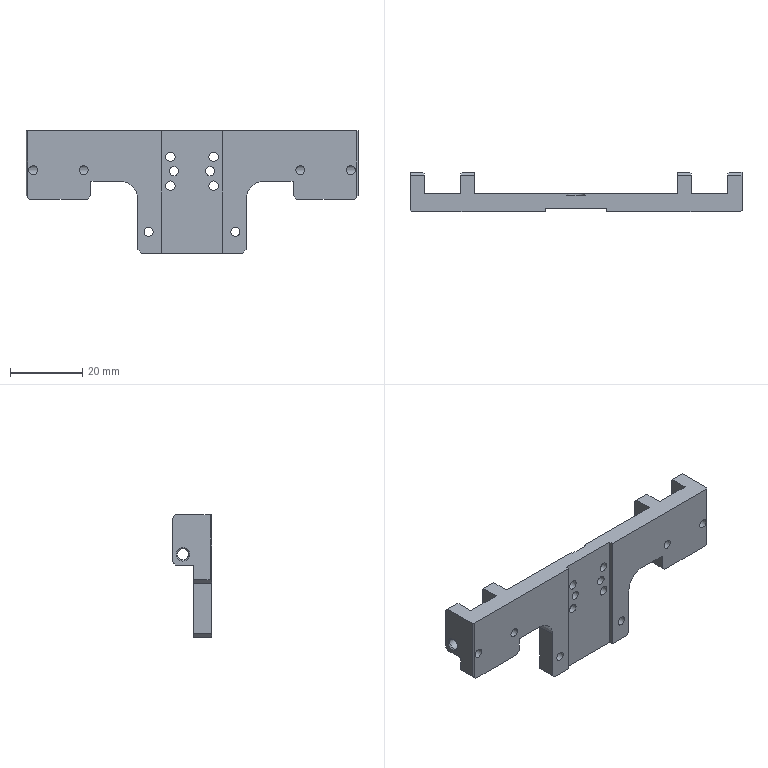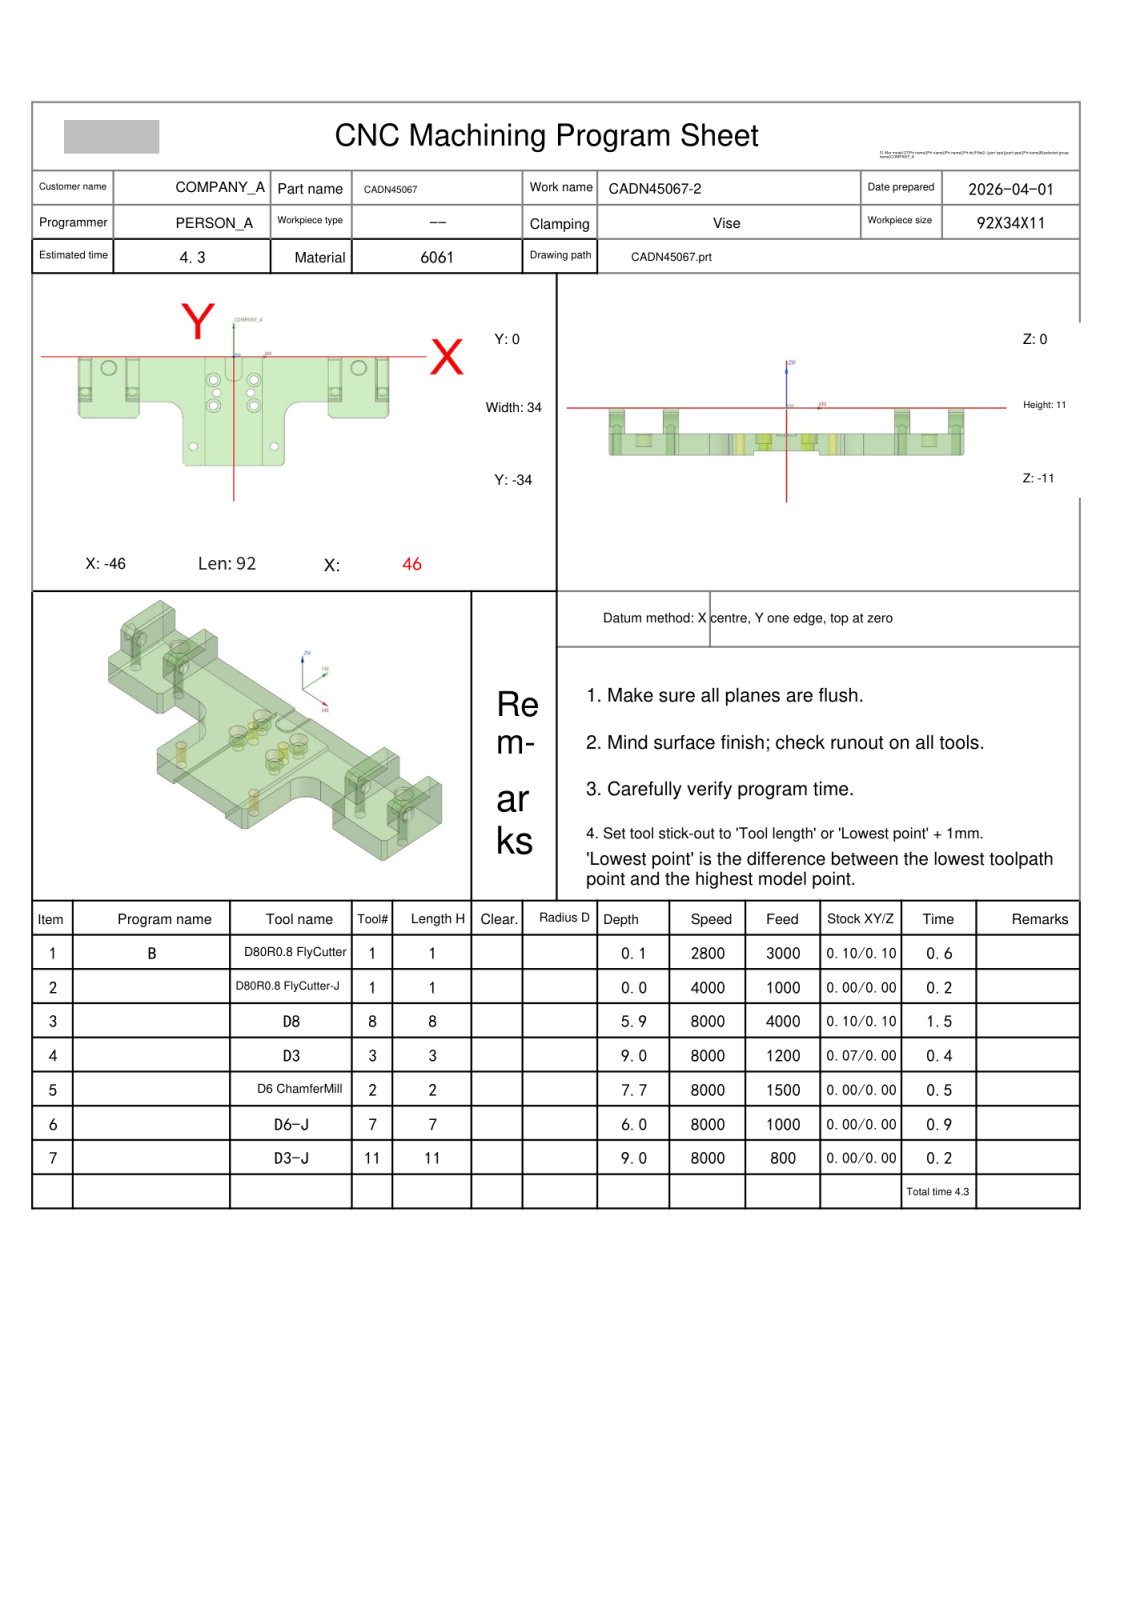NC program | NX | posted by the shop | part box 92 x 11 x 34 mm
Whole program:
%
O0001
(Machine time: 5.66 MIN)
(===Total Tool:6===)
(T1=D80R0.8 FlyCutter D=80.  R=0.8  D-  H01 Z=0.    )
(T8=D8      D=8.   R=0.   D-  H08 Z=-5.9  )
(T3=D3      D=3.   R=0.   D-  H03 Z=-9.   )
(T2=D6 ChamferMill   D=6.   R=0.   D-  H02 Z=-7.75 )
(T7=D6-J    D=6.   R=0.   D7  H07 Z=-6.   )
(T11=D3-J   D=3.   R=0.   D11 H11 Z=-9.   )
G80 G90 G17 G49 G40
G91 G28 Z0
M01
N1 T01 M06
(D80R0.8 FlyCutter  D=80. R=0.8 H=01 ce=0.10 di=0.10)
G00 G90 G54 X-98.097 Y-17. M03 S2800
G43 H01 Z20.
M08
Z5.014
G01 Z3.014 F3000.
X-86.097
X86.097
X98.097
Z5.014
G00 X-98.097
Z4.529
G01 Z2.529
X-86.097
X86.097
X98.097
Z4.529
G00 X-98.097
Z4.043
G01 Z2.043
X-86.097
X86.097
X98.097
Z4.043
G00 X-98.097
Z3.557
G01 Z1.557
X-86.097
X86.097
X98.097
Z3.557
G00 Z20.
X-98.097
Z3.071
G01 Z1.071
X-86.097
X86.097
X98.097
Z3.071
G00 Z20.
X-98.097
Z2.586
G01 Z.586
X-86.097
X86.097
X98.097
Z2.586
G00 Z20.
X-98.097
Z2.1
G01 Z.1
X-86.097
X86.097
X98.097
Z2.1
G00 Z20.
G91 G28 Z0.0
M05
M09
G91 G28 Z0.0
M01
N2 T01 M06
(D80R0.8 FlyCutter-J  D=80. R=0.8 H=01 ce=0.00 di=0.00)
G00 G90 G54 X-97.999 Y-17. M03 S4000
G43 H01 Z20.
M08
Z2.
G01 Z0.0 F1000.
X-85.999
X85.999
X97.999
Z2.
G00 Z20.
G91 G28 Z0.0
M05
M09
G91 G28 Z0.0
M01
N3 T08 M06
(D8  D=8. R=0. H=08 ce=0.10 di=0.10)
G00 G90 G54 X0.0 Y7. M03 S8000
G43 H08 Z13.5
M08
Z.91
G01 Z-.59 F4000.
Y3.92
X23.9
Y-18.1
X36.1
Y3.92
X37.9
Y-18.1
X49.92
Y-19.624
X46.624 Y-22.92
X28.609
X18.92 Y-26.933
Y-34.624
X15.624 Y-37.92
X-15.624
X-18.92 Y-34.624
Y-26.933
X-28.608 Y-22.92
X-46.624
X-49.92 Y-19.624
Y-18.1
X-37.9
Y3.92
X-36.1
Y-18.1
X-23.9
Y3.92
X-2.428
G02 X-1.763 Y3.564 I0.0 J-.8
G01 X1.763 Y-1.724
G03 X2.428 Y-2.08 I.665 J.444
G01 X17.102
G02 X17.9 Y-2.878 I-.002 J-.8
G01 Y-18.1
G03 X18.191 Y-19.947 I6. J0.0
G02 X18.229 Y-20.191 I-.762 J-.244
X17.738 Y-20.929 I-.8 J0.0
G01 X16.624 Y-21.39
G03 X12.92 Y-26.933 I2.296 J-5.543
G01 Y-31.122
G02 X12.122 Y-31.92 I-.8 J.002
G01 X-12.122
G02 X-12.92 Y-31.122 I.002 J.8
G01 Y-26.933
G03 X-16.624 Y-21.39 I-6. J0.0
G01 X-17.738 Y-20.929
G02 X-18.229 Y-20.191 I.308 J.738
X-18.191 Y-19.947 I.8 J0.0
G03 X-17.9 Y-18.1 I-5.709 J1.847
G01 Y-2.878
G02 X-17.102 Y-2.08 I.8 J-.002
G01 X-2.428
G02 X-1.763 Y-2.436 I0.0 J-.8
G01 X1.763 Y-7.724
G03 X2.428 Y-8.08 I.665 J.444
G01 X11.103
G02 X11.9 Y-8.877 I-.003 J-.8
G01 Y-16.802
G02 X11.591 Y-17.432 I-.8 J.003
G03 X7.041 Y-25.236 I7.329 J-9.502
G02 X6.252 Y-25.92 I-.792 J.116
G01 X-6.252
G02 X-7.041 Y-25.236 I.003 J.8
G03 X-11.591 Y-17.432 I-11.879 J-1.698
G02 X-11.9 Y-16.802 I.491 J.632
G01 Y-8.877
G02 X-11.103 Y-8.08 I.8 J-.003
G01 X-2.428
G02 X-1.763 Y-8.436 I0.0 J-.8
G01 X1.763 Y-13.724
G03 X2.428 Y-14.08 I.665 J.444
G01 X4.495
G02 X5.292 Y-14.88 I-.003 J-.8
X5.108 Y-15.391 I-.8 J0.0
G03 X2.547 Y-19.455 I13.812 J-11.542
G02 X1.823 Y-19.92 I-.727 J.335
G01 X-1.823
G02 X-2.547 Y-19.455 I.003 J.8
G03 X-5.108 Y-15.391 I-16.373 J-7.478
G02 X-5.292 Y-14.88 I.616 J.511
X-4.495 Y-14.08 I.8 J0.0
G01 X0.0
X.5
Y-11.08
Z.91
G00 X0.0 Y7.
Z.32
G01 Z-1.18
Y3.92
X23.9
Y-18.1
X36.1
Y3.92
X37.9
Y-18.1
X49.92
Y-19.624
X46.624 Y-22.92
X28.609
X18.92 Y-26.933
Y-34.624
X15.624 Y-37.92
X-15.624
X-18.92 Y-34.624
Y-26.933
X-28.608 Y-22.92
X-46.624
X-49.92 Y-19.624
Y-18.1
X-37.9
Y3.92
X-36.1
Y-18.1
X-23.9
Y3.92
X-2.428
G02 X-1.763 Y3.564 I0.0 J-.8
G01 X1.763 Y-1.724
G03 X2.428 Y-2.08 I.665 J.444
G01 X17.102
G02 X17.9 Y-2.878 I-.002 J-.8
G01 Y-18.1
G03 X18.191 Y-19.947 I6. J0.0
G02 X18.229 Y-20.191 I-.762 J-.244
X17.738 Y-20.929 I-.8 J0.0
G01 X16.624 Y-21.39
G03 X12.92 Y-26.933 I2.296 J-5.543
G01 Y-31.122
G02 X12.122 Y-31.92 I-.8 J.002
G01 X-12.122
G02 X-12.92 Y-31.122 I.002 J.8
G01 Y-26.933
G03 X-16.624 Y-21.39 I-6. J0.0
G01 X-17.738 Y-20.929
G02 X-18.229 Y-20.191 I.308 J.738
X-18.191 Y-19.947 I.8 J0.0
G03 X-17.9 Y-18.1 I-5.709 J1.847
G01 Y-2.878
G02 X-17.102 Y-2.08 I.8 J-.002
G01 X-2.428
G02 X-1.763 Y-2.436 I0.0 J-.8
G01 X1.763 Y-7.724
G03 X2.428 Y-8.08 I.665 J.444
G01 X11.103
G02 X11.9 Y-8.877 I-.003 J-.8
G01 Y-16.802
G02 X11.591 Y-17.432 I-.8 J.003
G03 X7.041 Y-25.236 I7.329 J-9.502
G02 X6.252 Y-25.92 I-.792 J.116
G01 X-6.252
G02 X-7.041 Y-25.236 I.003 J.8
G03 X-11.591 Y-17.432 I-11.879 J-1.698
G02 X-11.9 Y-16.802 I.491 J.632
G01 Y-8.877
G02 X-11.103 Y-8.08 I.8 J-.003
G01 X-2.428
G02 X-1.763 Y-8.436 I0.0 J-.8
G01 X1.763 Y-13.724
G03 X2.428 Y-14.08 I.665 J.444
G01 X4.495
G02 X5.292 Y-14.88 I-.003 J-.8
X5.108 Y-15.391 I-.8 J0.0
G03 X2.547 Y-19.455 I13.812 J-11.542
G02 X1.823 Y-19.92 I-.727 J.335
G01 X-1.823
G02 X-2.547 Y-19.455 I.003 J.8
G03 X-5.108 Y-15.391 I-16.373 J-7.478
G02 X-5.292 Y-14.88 I.616 J.511
X-4.495 Y-14.08 I.8 J0.0
G01 X0.0
X.5
Y-11.08
Z.32
G00 X0.0 Y7.
Z-.27
G01 Z-1.77
Y3.92
X23.9
Y-18.1
X36.1
Y3.92
X37.9
Y-18.1
X49.92
Y-19.624
X46.624 Y-22.92
X28.609
X18.92 Y-26.933
Y-34.624
X15.624 Y-37.92
X-15.624
X-18.92 Y-34.624
Y-26.933
X-28.608 Y-22.92
X-46.624
X-49.92 Y-19.624
Y-18.1
X-37.9
Y3.92
X-36.1
Y-18.1
X-23.9
Y3.92
X-2.428
G02 X-1.763 Y3.564 I0.0 J-.8
G01 X1.763 Y-1.724
G03 X2.428 Y-2.08 I.665 J.444
G01 X17.102
G02 X17.9 Y-2.878 I-.002 J-.8
G01 Y-18.1
G03 X18.191 Y-19.947 I6. J0.0
G02 X18.229 Y-20.191 I-.762 J-.244
X17.738 Y-20.929 I-.8 J0.0
G01 X16.624 Y-21.39
G03 X12.92 Y-26.933 I2.296 J-5.543
G01 Y-31.122
G02 X12.122 Y-31.92 I-.8 J.002
G01 X-12.122
G02 X-12.92 Y-31.122 I.002 J.8
G01 Y-26.933
G03 X-16.624 Y-21.39 I-6. J0.0
G01 X-17.738 Y-20.929
G02 X-18.229 Y-20.191 I.308 J.738
X-18.191 Y-19.947 I.8 J0.0
G03 X-17.9 Y-18.1 I-5.709 J1.847
G01 Y-2.878
G02 X-17.102 Y-2.08 I.8 J-.002
G01 X-2.428
G02 X-1.763 Y-2.436 I0.0 J-.8
G01 X1.763 Y-7.724
G03 X2.428 Y-8.08 I.665 J.444
G01 X11.103
G02 X11.9 Y-8.877 I-.003 J-.8
G01 Y-16.802
G02 X11.591 Y-17.432 I-.8 J.003
G03 X7.041 Y-25.236 I7.329 J-9.502
G02 X6.252 Y-25.92 I-.792 J.116
G01 X-6.252
G02 X-7.041 Y-25.236 I.003 J.8
G03 X-11.591 Y-17.432 I-11.879 J-1.698
G02 X-11.9 Y-16.802 I.491 J.632
G01 Y-8.877
G02 X-11.103 Y-8.08 I.8 J-.003
G01 X-2.428
G02 X-1.763 Y-8.436 I0.0 J-.8
G01 X1.763 Y-13.724
G03 X2.428 Y-14.08 I.665 J.444
G01 X4.495
G02 X5.292 Y-14.88 I-.003 J-.8
X5.108 Y-15.391 I-.8 J0.0
G03 X2.547 Y-19.455 I13.812 J-11.542
G02 X1.823 Y-19.92 I-.727 J.335
G01 X-1.823
G02 X-2.547 Y-19.455 I.003 J.8
G03 X-5.108 Y-15.391 I-16.373 J-7.478
G02 X-5.292 Y-14.88 I.616 J.511
X-4.495 Y-14.08 I.8 J0.0
G01 X0.0
X.5
Y-11.08
Z-.27
G00 X0.0 Y7.
Z-.86
G01 Z-2.36
Y3.92
X23.9
Y-18.1
X36.1
Y3.92
X37.9
Y-18.1
X49.92
Y-19.624
X46.624 Y-22.92
X28.609
X18.92 Y-26.933
Y-34.624
X15.624 Y-37.92
X-15.624
X-18.92 Y-34.624
Y-26.933
X-28.608 Y-22.92
X-46.624
X-49.92 Y-19.624
Y-18.1
X-37.9
Y3.92
X-36.1
Y-18.1
X-23.9
Y3.92
X-2.428
G02 X-1.763 Y3.564 I0.0 J-.8
G01 X1.763 Y-1.724
G03 X2.428 Y-2.08 I.665 J.444
G01 X17.102
G02 X17.9 Y-2.878 I-.002 J-.8
G01 Y-18.1
G03 X18.191 Y-19.947 I6. J0.0
G02 X18.229 Y-20.191 I-.762 J-.244
X17.738 Y-20.929 I-.8 J0.0
G01 X16.624 Y-21.39
G03 X12.92 Y-26.933 I2.296 J-5.543
G01 Y-31.122
G02 X12.122 Y-31.92 I-.8 J.002
G01 X-12.122
G02 X-12.92 Y-31.122 I.002 J.8
G01 Y-26.933
G03 X-16.624 Y-21.39 I-6. J0.0
G01 X-17.738 Y-20.929
G02 X-18.229 Y-20.191 I.308 J.738
X-18.191 Y-19.947 I.8 J0.0
G03 X-17.9 Y-18.1 I-5.709 J1.847
G01 Y-2.878
G02 X-17.102 Y-2.08 I.8 J-.002
G01 X-2.428
G02 X-1.763 Y-2.436 I0.0 J-.8
G01 X1.763 Y-7.724
G03 X2.428 Y-8.08 I.665 J.444
G01 X11.103
G02 X11.9 Y-8.877 I-.003 J-.8
G01 Y-16.802
G02 X11.591 Y-17.432 I-.8 J.003
G03 X7.041 Y-25.236 I7.329 J-9.502
G02 X6.252 Y-25.92 I-.792 J.116
G01 X-6.252
G02 X-7.041 Y-25.236 I.003 J.8
G03 X-11.591 Y-17.432 I-11.879 J-1.698
G02 X-11.9 Y-16.802 I.491 J.632
G01 Y-8.877
G02 X-11.103 Y-8.08 I.8 J-.003
G01 X-2.428
G02 X-1.763 Y-8.436 I0.0 J-.8
G01 X1.763 Y-13.724
G03 X2.428 Y-14.08 I.665 J.444
G01 X4.495
G02 X5.292 Y-14.88 I-.003 J-.8
X5.108 Y-15.391 I-.8 J0.0
G03 X2.547 Y-19.455 I13.812 J-11.542
G02 X1.823 Y-19.92 I-.727 J.335
G01 X-1.823
G02 X-2.547 Y-19.455 I.003 J.8
G03 X-5.108 Y-15.391 I-16.373 J-7.478
G02 X-5.292 Y-14.88 I.616 J.511
X-4.495 Y-14.08 I.8 J0.0
G01 X0.0
X.5
Y-11.08
Z-.86
G00 X0.0 Y7.
Z-1.45
G01 Z-2.95
Y3.92
X23.9
Y-18.1
X36.1
Y3.92
X37.9
Y-18.1
X49.92
Y-19.624
X46.624 Y-22.92
X28.609
X18.92 Y-26.933
Y-34.624
X15.624 Y-37.92
X-15.624
X-18.92 Y-34.624
Y-26.933
X-28.608 Y-22.92
X-46.624
X-49.92 Y-19.624
Y-18.1
X-37.9
Y3.92
X-36.1
Y-18.1
X-23.9
Y3.92
X-2.428
G02 X-1.763 Y3.564 I0.0 J-.8
G01 X1.763 Y-1.724
G03 X2.428 Y-2.08 I.665 J.444
G01 X17.102
G02 X17.9 Y-2.878 I-.002 J-.8
G01 Y-18.1
G03 X18.191 Y-19.947 I6. J0.0
G02 X18.229 Y-20.191 I-.762 J-.244
X17.738 Y-20.929 I-.8 J0.0
G01 X16.624 Y-21.39
G03 X12.92 Y-26.933 I2.296 J-5.543
G01 Y-31.122
G02 X12.122 Y-31.92 I-.8 J.002
G01 X-12.122
G02 X-12.92 Y-31.122 I.002 J.8
G01 Y-26.933
G03 X-16.624 Y-21.39 I-6. J0.0
G01 X-17.738 Y-20.929
G02 X-18.229 Y-20.191 I.308 J.738
X-18.191 Y-19.947 I.8 J0.0
G03 X-17.9 Y-18.1 I-5.709 J1.847
G01 Y-2.878
G02 X-17.102 Y-2.08 I.8 J-.002
G01 X-2.428
G02 X-1.763 Y-2.436 I0.0 J-.8
G01 X1.763 Y-7.724
G03 X2.428 Y-8.08 I.665 J.444
G01 X11.103
G02 X11.9 Y-8.877 I-.003 J-.8
G01 Y-16.802
G02 X11.591 Y-17.432 I-.8 J.003
G03 X7.041 Y-25.236 I7.329 J-9.502
G02 X6.252 Y-25.92 I-.792 J.116
G01 X-6.252
G02 X-7.041 Y-25.236 I.003 J.8
G03 X-11.591 Y-17.432 I-11.879 J-1.698
G02 X-11.9 Y-16.802 I.491 J.632
G01 Y-8.877
G02 X-11.103 Y-8.08 I.8 J-.003
G01 X-2.428
G02 X-1.763 Y-8.436 I0.0 J-.8
G01 X1.763 Y-13.724
G03 X2.428 Y-14.08 I.665 J.444
G01 X4.495
G02 X5.292 Y-14.88 I-.003 J-.8
X5.108 Y-15.391 I-.8 J0.0
G03 X2.547 Y-19.455 I13.812 J-11.542
G02 X1.823 Y-19.92 I-.727 J.335
G01 X-1.823
G02 X-2.547 Y-19.455 I.003 J.8
G03 X-5.108 Y-15.391 I-16.373 J-7.478
G02 X-5.292 Y-14.88 I.616 J.511
X-4.495 Y-14.08 I.8 J0.0
G01 X0.0
X.5
Y-11.08
Z-1.45
G00 X0.0 Y7.
Z-2.04
G01 Z-3.54
Y3.92
X23.9
Y-18.1
X36.1
Y3.92
X37.9
Y-18.1
X49.92
Y-19.624
X46.624 Y-22.92
X28.609
X18.92 Y-26.933
Y-34.624
X15.624 Y-37.92
X-15.624
X-18.92 Y-34.624
Y-26.933
X-28.608 Y-22.92
X-46.624
X-49.92 Y-19.624
Y-18.1
X-37.9
Y3.92
X-36.1
Y-18.1
X-23.9
Y3.92
X-2.428
G02 X-1.763 Y3.564 I0.0 J-.8
G01 X1.763 Y-1.724
G03 X2.428 Y-2.08 I.665 J.444
G01 X17.102
G02 X17.9 Y-2.878 I-.002 J-.8
G01 Y-18.1
G03 X18.191 Y-19.947 I6. J0.0
G02 X18.229 Y-20.191 I-.762 J-.244
X17.738 Y-20.929 I-.8 J0.0
G01 X16.624 Y-21.39
G03 X12.92 Y-26.933 I2.296 J-5.543
G01 Y-31.122
G02 X12.122 Y-31.92 I-.8 J.002
G01 X-12.122
G02 X-12.92 Y-31.122 I.002 J.8
G01 Y-26.933
G03 X-16.624 Y-21.39 I-6. J0.0
G01 X-17.738 Y-20.929
G02 X-18.229 Y-20.191 I.308 J.738
X-18.191 Y-19.947 I.8 J0.0
G03 X-17.9 Y-18.1 I-5.709 J1.847
G01 Y-2.878
G02 X-17.102 Y-2.08 I.8 J-.002
G01 X-2.428
G02 X-1.763 Y-2.436 I0.0 J-.8
G01 X1.763 Y-7.724
G03 X2.428 Y-8.08 I.665 J.444
G01 X11.103
G02 X11.9 Y-8.877 I-.003 J-.8
G01 Y-16.802
G02 X11.591 Y-17.432 I-.8 J.003
G03 X7.041 Y-25.236 I7.329 J-9.502
G02 X6.252 Y-25.92 I-.792 J.116
G01 X-6.252
G02 X-7.041 Y-25.236 I.003 J.8
G03 X-11.591 Y-17.432 I-11.879 J-1.698
G02 X-11.9 Y-16.802 I.491 J.632
G01 Y-8.877
G02 X-11.103 Y-8.08 I.8 J-.003
G01 X-2.428
G02 X-1.763 Y-8.436 I0.0 J-.8
G01 X1.763 Y-13.724
G03 X2.428 Y-14.08 I.665 J.444
G01 X4.495
G02 X5.292 Y-14.88 I-.003 J-.8
X5.108 Y-15.391 I-.8 J0.0
G03 X2.547 Y-19.455 I13.812 J-11.542
G02 X1.823 Y-19.92 I-.727 J.335
G01 X-1.823
G02 X-2.547 Y-19.455 I.003 J.8
G03 X-5.108 Y-15.391 I-16.373 J-7.478
G02 X-5.292 Y-14.88 I.616 J.511
X-4.495 Y-14.08 I.8 J0.0
G01 X0.0
X.5
Y-11.08
Z-2.04
G00 X0.0 Y7.
Z-2.63
G01 Z-4.13
Y3.92
X23.9
Y-18.1
X36.1
Y3.92
X37.9
Y-18.1
X49.92
Y-19.624
X46.624 Y-22.92
X28.609
X18.92 Y-26.933
Y-34.624
X15.624 Y-37.92
X-15.624
X-18.92 Y-34.624
Y-26.933
X-28.608 Y-22.92
X-46.624
X-49.92 Y-19.624
Y-18.1
X-37.9
Y3.92
X-36.1
Y-18.1
X-23.9
Y3.92
X-2.428
G02 X-1.763 Y3.564 I0.0 J-.8
G01 X1.763 Y-1.724
G03 X2.428 Y-2.08 I.665 J.444
G01 X17.102
G02 X17.9 Y-2.878 I-.002 J-.8
G01 Y-18.1
G03 X18.191 Y-19.947 I6. J0.0
G02 X18.229 Y-20.191 I-.762 J-.244
X17.738 Y-20.929 I-.8 J0.0
G01 X16.624 Y-21.39
G03 X12.92 Y-26.933 I2.296 J-5.543
G01 Y-31.122
G02 X12.122 Y-31.92 I-.8 J.002
G01 X-12.122
G02 X-12.92 Y-31.122 I.002 J.8
G01 Y-26.933
G03 X-16.624 Y-21.39 I-6. J0.0
G01 X-17.738 Y-20.929
G02 X-18.229 Y-20.191 I.308 J.738
X-18.191 Y-19.947 I.8 J0.0
G03 X-17.9 Y-18.1 I-5.709 J1.847
G01 Y-2.878
G02 X-17.102 Y-2.08 I.8 J-.002
G01 X-2.428
G02 X-1.763 Y-2.436 I0.0 J-.8
G01 X1.763 Y-7.724
G03 X2.428 Y-8.08 I.665 J.444
G01 X11.103
G02 X11.9 Y-8.877 I-.003 J-.8
G01 Y-16.802
G02 X11.591 Y-17.432 I-.8 J.003
G03 X7.041 Y-25.236 I7.329 J-9.502
G02 X6.252 Y-25.92 I-.792 J.116
G01 X-6.252
G02 X-7.041 Y-25.236 I.003 J.8
G03 X-11.591 Y-17.432 I-11.879 J-1.698
G02 X-11.9 Y-16.802 I.491 J.632
G01 Y-8.877
G02 X-11.103 Y-8.08 I.8 J-.003
G01 X-2.428
G02 X-1.763 Y-8.436 I0.0 J-.8
G01 X1.763 Y-13.724
G03 X2.428 Y-14.08 I.665 J.444
G01 X4.495
G02 X5.292 Y-14.88 I-.003 J-.8
X5.108 Y-15.391 I-.8 J0.0
G03 X2.547 Y-19.455 I13.812 J-11.542
G02 X1.823 Y-19.92 I-.727 J.335
G01 X-1.823
G02 X-2.547 Y-19.455 I.003 J.8
G03 X-5.108 Y-15.391 I-16.373 J-7.478
G02 X-5.292 Y-14.88 I.616 J.511
X-4.495 Y-14.08 I.8 J0.0
G01 X0.0
X.5
Y-11.08
Z-2.63
G00 X0.0 Y7.
Z-3.22
G01 Z-4.72
Y3.92
X23.9
Y-18.1
X36.1
Y3.92
X37.9
Y-18.1
X49.92
Y-19.624
X46.624 Y-22.92
X28.609
X18.92 Y-26.933
Y-34.624
X15.624 Y-37.92
X-15.624
X-18.92 Y-34.624
Y-26.933
X-28.608 Y-22.92
X-46.624
X-49.92 Y-19.624
Y-18.1
X-37.9
Y3.92
X-36.1
Y-18.1
X-23.9
Y3.92
X-2.428
G02 X-1.763 Y3.564 I0.0 J-.8
G01 X1.763 Y-1.724
G03 X2.428 Y-2.08 I.665 J.444
G01 X17.102
G02 X17.9 Y-2.878 I-.002 J-.8
G01 Y-18.1
G03 X18.191 Y-19.947 I6. J0.0
G02 X18.229 Y-20.191 I-.762 J-.244
X17.738 Y-20.929 I-.8 J0.0
G01 X16.624 Y-21.39
G03 X12.92 Y-26.933 I2.296 J-5.543
G01 Y-31.122
G02 X12.122 Y-31.92 I-.8 J.002
G01 X-12.122
G02 X-12.92 Y-31.122 I.002 J.8
G01 Y-26.933
G03 X-16.624 Y-21.39 I-6. J0.0
G01 X-17.738 Y-20.929
G02 X-18.229 Y-20.191 I.308 J.738
X-18.191 Y-19.947 I.8 J0.0
G03 X-17.9 Y-18.1 I-5.709 J1.847
G01 Y-2.878
G02 X-17.102 Y-2.08 I.8 J-.002
G01 X-2.428
G02 X-1.763 Y-2.436 I0.0 J-.8
G01 X1.763 Y-7.724
G03 X2.428 Y-8.08 I.665 J.444
G01 X11.103
G02 X11.9 Y-8.877 I-.003 J-.8
G01 Y-16.802
G02 X11.591 Y-17.432 I-.8 J.003
G03 X7.041 Y-25.236 I7.329 J-9.502
G02 X6.252 Y-25.92 I-.792 J.116
G01 X-6.252
G02 X-7.041 Y-25.236 I.003 J.8
G03 X-11.591 Y-17.432 I-11.879 J-1.698
G02 X-11.9 Y-16.802 I.491 J.632
G01 Y-8.877
G02 X-11.103 Y-8.08 I.8 J-.003
G01 X-2.428
G02 X-1.763 Y-8.436 I0.0 J-.8
G01 X1.763 Y-13.724
G03 X2.428 Y-14.08 I.665 J.444
G01 X4.495
G02 X5.292 Y-14.88 I-.003 J-.8
X5.108 Y-15.391 I-.8 J0.0
G03 X2.547 Y-19.455 I13.812 J-11.542
G02 X1.823 Y-19.92 I-.727 J.335
G01 X-1.823
G02 X-2.547 Y-19.455 I.003 J.8
G03 X-5.108 Y-15.391 I-16.373 J-7.478
G02 X-5.292 Y-14.88 I.616 J.511
X-4.495 Y-14.08 I.8 J0.0
G01 X0.0
X.5
Y-11.08
Z-3.22
G00 X0.0 Y7.
Z-3.81
G01 Z-5.31
Y3.92
X23.9
Y-18.1
X36.1
Y3.92
X37.9
Y-18.1
X49.92
Y-19.624
X46.624 Y-22.92
X28.609
X18.92 Y-26.933
Y-34.624
X15.624 Y-37.92
X-15.624
X-18.92 Y-34.624
Y-26.933
X-28.608 Y-22.92
X-46.624
X-49.92 Y-19.624
Y-18.1
X-37.9
Y3.92
X-36.1
Y-18.1
X-23.9
Y3.92
X-2.428
G02 X-1.763 Y3.564 I0.0 J-.8
G01 X1.763 Y-1.724
G03 X2.428 Y-2.08 I.665 J.444
G01 X17.102
G02 X17.9 Y-2.878 I-.002 J-.8
G01 Y-18.1
G03 X18.191 Y-19.947 I6. J0.0
G02 X18.229 Y-20.191 I-.762 J-.244
X17.738 Y-20.929 I-.8 J0.0
G01 X16.624 Y-21.39
G03 X12.92 Y-26.933 I2.296 J-5.543
G01 Y-31.122
G02 X12.122 Y-31.92 I-.8 J.002
G01 X-12.122
G02 X-12.92 Y-31.122 I.002 J.8
G01 Y-26.933
G03 X-16.624 Y-21.39 I-6. J0.0
G01 X-17.738 Y-20.929
G02 X-18.229 Y-20.191 I.308 J.738
X-18.191 Y-19.947 I.8 J0.0
G03 X-17.9 Y-18.1 I-5.709 J1.847
G01 Y-2.878
G02 X-17.102 Y-2.08 I.8 J-.002
G01 X-2.428
G02 X-1.763 Y-2.436 I0.0 J-.8
G01 X1.763 Y-7.724
G03 X2.428 Y-8.08 I.665 J.444
G01 X11.103
G02 X11.9 Y-8.877 I-.003 J-.8
G01 Y-16.802
G02 X11.591 Y-17.432 I-.8 J.003
G03 X7.041 Y-25.236 I7.329 J-9.502
G02 X6.252 Y-25.92 I-.792 J.116
G01 X-6.252
G02 X-7.041 Y-25.236 I.003 J.8
G03 X-11.591 Y-17.432 I-11.879 J-1.698
G02 X-11.9 Y-16.802 I.491 J.632
G01 Y-8.877
G02 X-11.103 Y-8.08 I.8 J-.003
G01 X-2.428
G02 X-1.763 Y-8.436 I0.0 J-.8
G01 X1.763 Y-13.724
G03 X2.428 Y-14.08 I.665 J.444
G01 X4.495
G02 X5.292 Y-14.88 I-.003 J-.8
X5.108 Y-15.391 I-.8 J0.0
G03 X2.547 Y-19.455 I13.812 J-11.542
G02 X1.823 Y-19.92 I-.727 J.335
G01 X-1.823
G02 X-2.547 Y-19.455 I.003 J.8
G03 X-5.108 Y-15.391 I-16.373 J-7.478
G02 X-5.292 Y-14.88 I.616 J.511
X-4.495 Y-14.08 I.8 J0.0
G01 X0.0
X.5
Y-11.08
Z-3.81
G00 X0.0 Y7.
Z-4.4
G01 Z-5.9
Y3.92
X23.9
Y-18.1
X36.1
Y3.92
X37.9
Y-18.1
X49.92
Y-19.624
X46.624 Y-22.92
X28.609
X18.92 Y-26.933
Y-34.624
X15.624 Y-37.92
X-15.624
X-18.92 Y-34.624
Y-26.933
X-28.608 Y-22.92
X-46.624
X-49.92 Y-19.624
Y-18.1
X-37.9
Y3.92
X-36.1
Y-18.1
X-23.9
Y3.92
X-2.428
G02 X-1.763 Y3.564 I0.0 J-.8
G01 X1.763 Y-1.724
G03 X2.428 Y-2.08 I.665 J.444
G01 X17.102
G02 X17.9 Y-2.878 I-.002 J-.8
G01 Y-18.1
G03 X18.191 Y-19.947 I6. J0.0
G02 X18.229 Y-20.191 I-.762 J-.244
X17.738 Y-20.929 I-.8 J0.0
G01 X16.624 Y-21.39
G03 X12.92 Y-26.933 I2.296 J-5.543
G01 Y-31.122
G02 X12.122 Y-31.92 I-.8 J.002
G01 X-12.122
G02 X-12.92 Y-31.122 I.002 J.8
G01 Y-26.933
G03 X-16.624 Y-21.39 I-6. J0.0
G01 X-17.738 Y-20.929
G02 X-18.229 Y-20.191 I.308 J.738
X-18.191 Y-19.947 I.8 J0.0
G03 X-17.9 Y-18.1 I-5.709 J1.847
G01 Y-2.878
G02 X-17.102 Y-2.08 I.8 J-.002
G01 X-2.428
G02 X-1.763 Y-2.436 I0.0 J-.8
G01 X1.763 Y-7.724
G03 X2.428 Y-8.08 I.665 J.444
G01 X11.103
G02 X11.9 Y-8.877 I-.003 J-.8
G01 Y-16.802
G02 X11.591 Y-17.432 I-.8 J.003
G03 X7.041 Y-25.236 I7.329 J-9.502
G02 X6.252 Y-25.92 I-.792 J.116
G01 X-6.252
G02 X-7.041 Y-25.236 I.003 J.8
G03 X-11.591 Y-17.432 I-11.879 J-1.698
G02 X-11.9 Y-16.802 I.491 J.632
G01 Y-8.877
G02 X-11.103 Y-8.08 I.8 J-.003
G01 X-2.428
G02 X-1.763 Y-8.436 I0.0 J-.8
G01 X1.763 Y-13.724
G03 X2.428 Y-14.08 I.665 J.444
G01 X4.495
G02 X5.292 Y-14.88 I-.003 J-.8
X5.108 Y-15.391 I-.8 J0.0
G03 X2.547 Y-19.455 I13.812 J-11.542
G02 X1.823 Y-19.92 I-.727 J.335
G01 X-1.823
G02 X-2.547 Y-19.455 I.003 J.8
G03 X-5.108 Y-15.391 I-16.373 J-7.478
G02 X-5.292 Y-14.88 I.616 J.511
X-4.495 Y-14.08 I.8 J0.0
G01 X0.0
X.5
Y-11.08
Z-4.4
G00 Z13.5
G91 G28 Z0.0
M05
M09
G91 G28 Z0.0
M01
N4 T03 M06
(D3  D=3. R=0. H=03 ce=0.10 di=0.00)
G00 G90 G54 X37. Y-3.5 M03 S8000
G43 H03 Z20.
M08
Z-5.4
G03 X36.75 Y-3.25 I-.25 J0.0 F1100.
X36.5 Y-3.5 I0.0 J-.25
X36.5 Y-3.5 Z-5.6 I.5 J0.0
X36.5 Y-3.5 Z-5.8 I.5 J0.0
X36.5 Y-3.5 Z-6. I.5 J0.0
X36.5 Y-3.5 Z-6.2 I.5 J0.0
X36.5 Y-3.5 Z-6.4 I.5 J0.0
X36.5 Y-3.5 Z-6.6 I.5 J0.0
X36.5 Y-3.5 Z-6.8 I.5 J0.0
X36.5 Y-3.5 Z-7. I.5 J0.0
X36.5 Y-3.5 Z-7.2 I.5 J0.0
X36.5 Y-3.5 Z-7.4 I.5 J0.0
X36.5 Y-3.5 Z-7.6 I.5 J0.0
X36.5 Y-3.5 Z-7.8 I.5 J0.0
X36.5 Y-3.5 Z-8. I.5 J0.0
X36.5 Y-3.5 Z-8.2 I.5 J0.0
X36.5 Y-3.5 Z-8.4 I.5 J0.0
X36.5 Y-3.5 Z-8.6 I.5 J0.0
X36.5 Y-3.5 Z-8.8 I.5 J0.0
X36.5 Y-3.5 Z-9. I.5 J0.0
X37. Y-4. I.5 J0.0
X37.5 Y-3.5 I0.0 J.5
X37. Y-3. I-.5 J0.0
X36.5 Y-3.5 I0.0 J-.5
X36.75 Y-3.75 I.25 J0.0
X37. Y-3.5 I0.0 J.25
G00 Z20.
X-37.
Z-5.4
G03 X-37.25 Y-3.25 I-.25 J0.0
X-37.5 Y-3.5 I0.0 J-.25
X-37.5 Y-3.5 Z-5.6 I.5 J0.0
X-37.5 Y-3.5 Z-5.8 I.5 J0.0
X-37.5 Y-3.5 Z-6. I.5 J0.0
X-37.5 Y-3.5 Z-6.2 I.5 J0.0
X-37.5 Y-3.5 Z-6.4 I.5 J0.0
X-37.5 Y-3.5 Z-6.6 I.5 J0.0
X-37.5 Y-3.5 Z-6.8 I.5 J0.0
X-37.5 Y-3.5 Z-7. I.5 J0.0
X-37.5 Y-3.5 Z-7.2 I.5 J0.0
X-37.5 Y-3.5 Z-7.4 I.5 J0.0
X-37.5 Y-3.5 Z-7.6 I.5 J0.0
X-37.5 Y-3.5 Z-7.8 I.5 J0.0
X-37.5 Y-3.5 Z-8. I.5 J0.0
X-37.5 Y-3.5 Z-8.2 I.5 J0.0
X-37.5 Y-3.5 Z-8.4 I.5 J0.0
X-37.5 Y-3.5 Z-8.6 I.5 J0.0
X-37.5 Y-3.5 Z-8.8 I.5 J0.0
X-37.5 Y-3.5 Z-9. I.5 J0.0
X-37. Y-4. I.5 J0.0
X-36.5 Y-3.5 I0.0 J.5
X-37. Y-3. I-.5 J0.0
X-37.5 Y-3.5 I0.0 J-.5
X-37.25 Y-3.75 I.25 J0.0
X-37. Y-3.5 I0.0 J.25
G00 Z20.
G00 G90 X6. Y-7.25 M03 S8000
Z20.
Z-5.7
G03 X5.71 Y-6.96 I-.29 J0.0 F1200.
X5.42 Y-7.25 I0.0 J-.29
X5.42 Y-7.25 Z-5.9 I.58 J0.0
X5.42 Y-7.25 Z-6.1 I.58 J0.0
X5.42 Y-7.25 Z-6.3 I.58 J0.0
X5.42 Y-7.25 Z-6.5 I.58 J0.0
X5.42 Y-7.25 Z-6.7 I.58 J0.0
X5.42 Y-7.25 Z-6.9 I.58 J0.0
X5.42 Y-7.25 Z-7.1 I.58 J0.0
X5.42 Y-7.25 Z-7.3 I.58 J0.0
X5.42 Y-7.25 Z-7.5 I.58 J0.0
X5.42 Y-7.25 Z-7.7 I.58 J0.0
X5.42 Y-7.25 Z-7.9 I.58 J0.0
X5.42 Y-7.25 Z-8.1 I.58 J0.0
X5.42 Y-7.25 Z-8.3 I.58 J0.0
X6. Y-7.83 I.58 J0.0
X6.58 Y-7.25 I0.0 J.58
X6. Y-6.67 I-.58 J0.0
X5.42 Y-7.25 I0.0 J-.58
X5.71 Y-7.54 I.29 J0.0
X6. Y-7.25 I0.0 J.29
G00 Z20.
Y-15.25
Z-5.7
G03 X5.71 Y-14.96 I-.29 J0.0
X5.42 Y-15.25 I0.0 J-.29
X5.42 Y-15.25 Z-5.9 I.58 J0.0
X5.42 Y-15.25 Z-6.1 I.58 J0.0
X5.42 Y-15.25 Z-6.3 I.58 J0.0
X5.42 Y-15.25 Z-6.5 I.58 J0.0
X5.42 Y-15.25 Z-6.7 I.58 J0.0
X5.42 Y-15.25 Z-6.9 I.58 J0.0
X5.42 Y-15.25 Z-7.1 I.58 J0.0
X5.42 Y-15.25 Z-7.3 I.58 J0.0
X5.42 Y-15.25 Z-7.5 I.58 J0.0
X5.42 Y-15.25 Z-7.7 I.58 J0.0
X5.42 Y-15.25 Z-7.9 I.58 J0.0
X5.42 Y-15.25 Z-8.1 I.58 J0.0
X5.42 Y-15.25 Z-8.3 I.58 J0.0
X6. Y-15.83 I.58 J0.0
X6.58 Y-15.25 I0.0 J.58
X6. Y-14.67 I-.58 J0.0
X5.42 Y-15.25 I0.0 J-.58
X5.71 Y-15.54 I.29 J0.0
X6. Y-15.25 I0.0 J.29
G00 Z20.
X-6.
Z-5.7
G03 X-6.29 Y-14.96 I-.29 J0.0
X-6.58 Y-15.25 I0.0 J-.29
X-6.58 Y-15.25 Z-5.9 I.58 J0.0
X-6.58 Y-15.25 Z-6.1 I.58 J0.0
X-6.58 Y-15.25 Z-6.3 I.58 J0.0
X-6.58 Y-15.25 Z-6.5 I.58 J0.0
X-6.58 Y-15.25 Z-6.7 I.58 J0.0
X-6.58 Y-15.25 Z-6.9 I.58 J0.0
X-6.58 Y-15.25 Z-7.1 I.58 J0.0
X-6.58 Y-15.25 Z-7.3 I.58 J0.0
X-6.58 Y-15.25 Z-7.5 I.58 J0.0
X-6.58 Y-15.25 Z-7.7 I.58 J0.0
X-6.58 Y-15.25 Z-7.9 I.58 J0.0
X-6.58 Y-15.25 Z-8.1 I.58 J0.0
X-6.58 Y-15.25 Z-8.3 I.58 J0.0
X-6. Y-15.83 I.58 J0.0
X-5.42 Y-15.25 I0.0 J.58
X-6. Y-14.67 I-.58 J0.0
X-6.58 Y-15.25 I0.0 J-.58
X-6.29 Y-15.54 I.29 J0.0
X-6. Y-15.25 I0.0 J.29
G00 Z20.
Y-7.25
Z-5.7
G03 X-6.29 Y-6.96 I-.29 J0.0
X-6.58 Y-7.25 I0.0 J-.29
X-6.58 Y-7.25 Z-5.9 I.58 J0.0
X-6.58 Y-7.25 Z-6.1 I.58 J0.0
X-6.58 Y-7.25 Z-6.3 I.58 J0.0
X-6.58 Y-7.25 Z-6.5 I.58 J0.0
X-6.58 Y-7.25 Z-6.7 I.58 J0.0
X-6.58 Y-7.25 Z-6.9 I.58 J0.0
X-6.58 Y-7.25 Z-7.1 I.58 J0.0
X-6.58 Y-7.25 Z-7.3 I.58 J0.0
X-6.58 Y-7.25 Z-7.5 I.58 J0.0
X-6.58 Y-7.25 Z-7.7 I.58 J0.0
X-6.58 Y-7.25 Z-7.9 I.58 J0.0
X-6.58 Y-7.25 Z-8.1 I.58 J0.0
X-6.58 Y-7.25 Z-8.3 I.58 J0.0
X-6. Y-7.83 I.58 J0.0
X-5.42 Y-7.25 I0.0 J.58
X-6. Y-6.67 I-.58 J0.0
X-6.58 Y-7.25 I0.0 J-.58
X-6.29 Y-7.54 I.29 J0.0
X-6. Y-7.25 I0.0 J.29
G00 Z20.
G00 G90 X-.9 Y4.6 M03 S8000
Z13.5
Z-4.7
G01 Z-6.2 F1000.
Y1.47
Y-5.5
G03 X-.5 Y-5.9 I.4 J0.0
G01 X.5
G03 X.9 Y-5.5 I0.0 J.4
G01 Y1.47
Y4.6
Z-4.7
G00 X-.9
Z-4.9
G01 Z-6.4
Y1.47
Y-5.5
G03 X-.5 Y-5.9 I.4 J0.0
G01 X.5
G03 X.9 Y-5.5 I0.0 J.4
G01 Y1.47
Y4.6
Z-4.9
G00 Z13.5
G91 G28 Z0.0
M05
M09
G91 G28 Z0.0
M01
N5 T02 M06
(D6 ChamferMill  D=6. R=0. H=02 ce=0.00 di=0.10)
G00 G90 G54 X12. Y-28. M03 S8000
G43 H02 Z20.
M08
G98 G81 X12. Y-28. Z-7.75 R-3. F1000.
X5. Y-11.25
X-5.
X-12. Y-28.
G80
G00 Z20.
G00 G90 X46.528 Y-.731 M03 S6500
Z20.
Z3.2
G01 Z-.8 F1500.
X46.571 Y-.815
X46.6 Y-1.
Y-7.
Y-13.
X46.571 Y-13.185
X46.528 Y-13.269
Z3.2
G00 Z10.
X27.472
Z3.2
G01 Z-.8
X27.429 Y-13.185
X27.4 Y-13.
Y-7.
Y-1.
X27.429 Y-.815
X27.472 Y-.731
Z3.2
G00 Z10.
X-27.472
Z3.2
G01 Z-.8
X-27.429 Y-.815
X-27.4 Y-1.
Y-7.
Y-13.
X-27.429 Y-13.185
X-27.472 Y-13.269
Z3.2
G00 Z10.
X-46.528
Z3.2
G01 Z-.8
X-46.571 Y-13.185
X-46.6 Y-13.
Y-7.
Y-1.
X-46.571 Y-.815
X-46.528 Y-.731
Z3.2
G00 Z10.
X-38.873 Y.668
Z-2.127
G01 Z-6.799
X-38.788 Y.608
X-38.758 Y.6
X-35.242
X-35.212 Y.608
X-35.127 Y.668
Z-2.127
G00 Z10.
X-27.355 Y-17.142
Z-2.13
G01 Z-6.799
X-27.395 Y-17.199
X-27.4 Y-17.219
Y-18.
X-27.42 Y-18.155
X-27.48 Y-18.3
X-27.576 Y-18.424
X-28.576 Y-19.424
X-28.7 Y-19.52
X-28.845 Y-19.58
X-29. Y-19.6
X-45.
X-45.155 Y-19.58
X-45.3 Y-19.52
X-45.424 Y-19.424
X-46.424 Y-18.424
X-46.52 Y-18.3
X-46.58 Y-18.155
X-46.6 Y-18.
Y-17.219
X-46.605 Y-17.199
X-46.645 Y-17.142
Z-2.13
G00 Z10.
X24.858 Y-14.645
Z-2.127
G01 Z-6.799
X24.801 Y-14.605
X24.781 Y-14.6
X20.
G03 X15.6 Y-19. I0.0 J-4.4
G01 Y-33.
X15.58 Y-33.155
X15.52 Y-33.3
X15.424 Y-33.424
X14.424 Y-34.424
X14.3 Y-34.52
X14.155 Y-34.58
X14. Y-34.6
X-14.
X-14.155 Y-34.58
X-14.3 Y-34.52
X-14.424 Y-34.424
X-15.424 Y-33.424
X-15.52 Y-33.3
X-15.58 Y-33.155
X-15.6 Y-33.
Y-19.
G03 X-20. Y-14.6 I-4.4 J0.0
G01 X-24.781
X-24.801 Y-14.605
X-24.858 Y-14.645
Z-2.127
G00 Z10.
X-24.878 Y.668
Z-2.127
G01 Z-6.799
X-24.793 Y.608
X-24.763 Y.6
X-2.5
X-2.315 Y.571
X-2.147 Y.485
X-2.015 Y.353
X-1.993 Y.311
X-1.982 Y.272
Z-2.799
G00 X1.956 Y.287
Z-5.217
G01 Z-6.799
X1.986 Y.303
X1.993 Y.311
X2.015 Y.353
X2.147 Y.485
X2.315 Y.571
X2.5 Y.6
X24.763
X24.793 Y.608
X24.878 Y.668
Z-2.127
G00 Z10.
X6.407 Y-5.885
Z-5.317
G01 Z-6.799
G03 X6.102 Y-5.716 I-1.118 J-1.658
G01 X6.054 Y-5.691
X6. Y-5.7
G03 X4.45 Y-7.25 I0.0 J-1.55
X6. Y-8.8 I1.55 J0.0
X7.55 Y-7.25 I0.0 J1.55
X6. Y-5.7 I-1.55 J0.0
G01 X5.946 Y-5.691
X5.898 Y-5.716
G03 X5.593 Y-5.885 I.813 J-1.827
G01 Z-5.317
G00 Z-3.049
X6.407 Y-13.885
Z-5.317
G01 Z-6.799
G03 X6.102 Y-13.716 I-1.118 J-1.658
G01 X6.054 Y-13.691
X6. Y-13.7
G03 X4.45 Y-15.25 I0.0 J-1.55
X6. Y-16.8 I1.55 J0.0
X7.55 Y-15.25 I0.0 J1.55
X6. Y-13.7 I-1.55 J0.0
G01 X5.946 Y-13.691
X5.898 Y-13.716
G03 X5.593 Y-13.885 I.813 J-1.827
G01 Z-5.317
G00 Z-3.049
X-5.593
Z-5.317
G01 Z-6.799
G03 X-5.898 Y-13.716 I-1.118 J-1.658
G01 X-5.946 Y-13.691
X-6. Y-13.7
G03 X-7.55 Y-15.25 I0.0 J-1.55
X-6. Y-16.8 I1.55 J0.0
X-4.45 Y-15.25 I0.0 J1.55
X-6. Y-13.7 I-1.55 J0.0
G01 X-6.054 Y-13.691
X-6.102 Y-13.716
G03 X-6.407 Y-13.885 I.813 J-1.827
G01 Z-5.317
G00 Z-3.049
X-5.593 Y-5.885
Z-5.317
G01 Z-6.799
G03 X-5.898 Y-5.716 I-1.118 J-1.658
G01 X-5.946 Y-5.691
X-6. Y-5.7
G03 X-7.55 Y-7.25 I0.0 J-1.55
X-6. Y-8.8 I1.55 J0.0
X-4.45 Y-7.25 I0.0 J1.55
X-6. Y-5.7 I-1.55 J0.0
G01 X-6.054 Y-5.691
X-6.102 Y-5.716
G03 X-6.407 Y-5.885 I.813 J-1.827
G01 Z-5.317
G00 Z10.
X35.127 Y.668
Z-2.127
G01 Z-6.799
X35.212 Y.608
X35.242 Y.6
X38.758
X38.788 Y.608
X38.873 Y.668
Z-2.127
G00 Z10.
X46.645 Y-17.142
Z-2.13
G01 Z-6.799
X46.605 Y-17.199
X46.6 Y-17.219
Y-18.
X46.58 Y-18.155
X46.52 Y-18.3
X46.424 Y-18.424
X45.424 Y-19.424
X45.3 Y-19.52
X45.155 Y-19.58
X45. Y-19.6
X29.
X28.845 Y-19.58
X28.7 Y-19.52
X28.576 Y-19.424
X27.576 Y-18.424
X27.48 Y-18.3
X27.42 Y-18.155
X27.4 Y-18.
Y-17.219
X27.395 Y-17.199
X27.355 Y-17.142
Z-2.13
G00 Z10.
X-1.367 Y.6
Z-3.299
G01 Z-7.299
X1.367
Z-3.299
G00 Z20.
G00 G90 X25.1 Y.708 M03 S6500
Z20.
Z-.2
G01 Z-1.7 F1500.
X25.168 Y.699
X25.237 Y.7
X33.2
Y-14.7
X25.237
X25.168 Y-14.699
X25.1 Y-14.708
Z-.2
G00 X48.9
G01 Z-1.7
X48.832 Y-14.699
X48.763 Y-14.7
X40.8
Y.7
X48.763
X48.832 Y.699
X48.9 Y.708
Z-.2
G00 Z20.
X37.197 Y-3.467
Z-5.5
G01 Z-7.
X38.2 Y-3.3
G03 X37. Y-2.1 I-1.2 J0.0
X35.6 Y-3.5 I0.0 J-1.4
X37. Y-4.9 I1.4 J0.0
X38.4 Y-3.5 I0.0 J1.4
X37. Y-2.1 I-1.4 J0.0
X36.605 Y-2.157 I0.0 J-1.4
X35.744 Y-3.308 I.338 J-1.151
X35.792 Y-3.646 I1.2 J0.0
G01 X36.801 Y-3.524
Z-5.5
G00 Z20.
X-25.1 Y-14.708
Z-.2
G01 Z-1.7
X-25.168 Y-14.699
X-25.237 Y-14.7
X-33.2
Y.7
X-25.237
X-25.168 Y.699
X-25.1 Y.708
Z-.2
G00 X-48.9
G01 Z-1.7
X-48.832 Y.699
X-48.763 Y.7
X-40.8
Y-14.7
X-48.763
X-48.832 Y-14.699
X-48.9 Y-14.708
Z-.2
G00 Z20.
X-36.803 Y-3.467
Z-5.5
G01 Z-7.
X-35.8 Y-3.3
G03 X-37. Y-2.1 I-1.2 J0.0
X-38.4 Y-3.5 I0.0 J-1.4
X-37. Y-4.9 I1.4 J0.0
X-35.6 Y-3.5 I0.0 J1.4
X-37. Y-2.1 I-1.4 J0.0
X-37.395 Y-2.157 I0.0 J-1.4
X-38.256 Y-3.308 I.338 J-1.151
X-38.208 Y-3.646 I1.2 J0.0
G01 X-37.199 Y-3.524
Z-5.5
G00 Z20.
G91 G28 Z0.0
M05
M09
G91 G28 Z0.0
M01
N6 T07 M06
(D6-J  D=6. R=0. H=07 ce=0.40 di=0.00)
G00 G90 G54 X38.2 Y-23.2 M03 S8000
G43 H07 Z13.5
M08
Z-4.5
G01 Z-6. F1000.
Y-20.8
G03 X37. Y-19.6 I-1.2 J0.0
G01 X28.998
G02 X28.577 Y-19.426 I.002 J.6
G01 X27.612 Y-18.46
X26.42 Y-17.617
X26.37 Y-17.52
X26.489 Y-17.4
X35.4
Y.002
G02 X35.998 Y.6 I.6 J-.002
G01 X38.002
G02 X38.6 Y.002 I-.002 J-.6
G01 Y-17.4
X46.002
G02 X46.6 Y-18. I-.002 J-.6
X46.426 Y-18.423 I-.6 J0.0
G01 X45.423 Y-19.426
G02 X45.002 Y-19.6 I-.423 J.426
G01 X37.
X36.
G03 X34.8 Y-20.8 I0.0 J-1.2
G01 Y-23.2
Z-4.5
G00 Z13.5
X-1.2 Y4.2
Z-4.5
G01 Z-6.
Y1.8
G03 X0.0 Y.6 I1.2 J0.0
G01 X24.002
G02 X24.6 Y.002 I-.002 J-.6
G01 Y-15.984
G02 X24.42 Y-16.162 I-.18 J.001
G01 X24.317 Y-16.13
X22.154 Y-14.6
X20.
G03 X15.6 Y-19. I0.0 J-4.4
G01 Y-33.002
G02 X15.426 Y-33.423 I-.6 J.002
G01 X14.423 Y-34.426
G02 X14.002 Y-34.6 I-.423 J.426
G01 X-14.002
G02 X-14.423 Y-34.426 I.002 J.6
G01 X-15.426 Y-33.423
G02 X-15.6 Y-33.002 I.426 J.423
G01 Y-19.
G03 X-20. Y-14.6 I-4.4 J0.0
G01 X-22.154
X-24.317 Y-16.13
X-24.42 Y-16.162
G02 X-24.6 Y-15.984 I0.0 J.18
G01 Y.002
G02 X-24.002 Y.6 I.6 J-.002
G01 X3.
G02 X3.565 Y.203 I0.0 J-.6
G01 X4.357 Y-2.003
G03 X4.922 Y-2.4 I.565 J.203
G01 X21.003
G02 X21.6 Y-2.997 I-.003 J-.6
G01 Y-11.003
G02 X21.003 Y-11.6 I-.6 J.003
G01 X20.
G03 X12.6 Y-19. I0.0 J-7.4
G01 Y-31.003
G02 X12.003 Y-31.6 I-.6 J.003
G01 X-12.003
G02 X-12.6 Y-31.003 I.003 J.6
G01 Y-19.
G03 X-20. Y-11.6 I-7.4 J0.0
G01 X-21.003
G02 X-21.6 Y-11.003 I.003 J.6
G01 Y-2.997
G02 X-21.003 Y-2.4 I.6 J-.003
G01 X1.252
G02 X1.676 Y-2.576 I0.0 J-.6
G01 X4.324 Y-5.224
G03 X4.748 Y-5.4 I.424 J.424
G01 X18.003
G02 X18.6 Y-5.997 I-.003 J-.6
G01 Y-8.186
G02 X18.112 Y-8.773 I-.6 J.003
G03 X9.6 Y-19. I1.888 J-10.227
G01 Y-28.003
G02 X9.003 Y-28.6 I-.6 J.003
G01 X-9.003
G02 X-9.6 Y-28.003 I.003 J.6
G01 Y-19.
G03 X-18.112 Y-8.773 I-10.4 J0.0
G02 X-18.6 Y-8.186 I.112 J.59
G01 Y-5.997
G02 X-18.003 Y-5.4 I.6 J-.003
G01 X1.252
G02 X1.676 Y-5.576 I0.0 J-.6
G01 X4.324 Y-8.224
G03 X4.748 Y-8.4 I.424 J.424
G01 X10.205
G02 X10.802 Y-9. I-.003 J-.6
X10.624 Y-9.427 I-.6 J0.0
G03 X6.6 Y-19. I9.376 J-9.573
G01 Y-25.003
G02 X6.003 Y-25.6 I-.6 J.003
G01 X-6.003
G02 X-6.6 Y-25.003 I.003 J.6
G01 Y-19.
G03 X-10.624 Y-9.427 I-13.4 J0.0
G02 X-10.802 Y-9. I.422 J.427
X-10.205 Y-8.4 I.6 J0.0
G01 X1.252
G02 X1.675 Y-8.575 I0.0 J-.6
G01 X4.37 Y-11.26
G03 X4.651 Y-11.417 I.423 J.425
G02 X5.108 Y-12. I-.142 J-.583
X5.056 Y-12.245 I-.6 J0.0
G03 X3.6 Y-19. I14.944 J-6.755
G01 Y-22.003
G02 X3.003 Y-22.6 I-.6 J.003
G01 X-3.003
G02 X-3.6 Y-22.003 I.003 J.6
G01 Y-19.
G03 X-5.056 Y-12.245 I-16.4 J0.0
G02 X-5.108 Y-12. I.548 J.245
X-4.511 Y-11.4 I.6 J0.0
G01 X.968
G02 X1.388 Y-11.82 I0.0 J-.42
G01 X1.376 Y-11.918
X.828 Y-14.209
X.812 Y-14.348
G03 X.908 Y-14.674 I.6 J0.0
G02 X1.004 Y-15. I-.504 J-.326
G01 X.993 Y-15.117
G03 X.6 Y-19. I19.007 J-3.883
G01 Y-19.003
G02 X0.0 Y-19.6 I-.6 J.003
G01 X-.003
G02 X-.6 Y-19.003 I.003 J.6
G01 Y-19.
G03 X-.993 Y-15.117 I-19.4 J0.0
G01 X-1.004 Y-15.
G02 X-.407 Y-14.4 I.6 J0.0
G01 X.407
G02 X.755 Y-14.513 I-.003 J-.6
X1.004 Y-15. I-.351 J-.487
G01 X.993 Y-15.117
G03 X.932 Y-15.426 I19.007 J-3.883
X.912 Y-15.647 I1.179 J-.221
X1.89 Y-16.826 I1.2 J0.0
G01 Z-4.5
G00 Z-2.
X-35.8 Y-23.2
Z-4.5
G01 Z-6.
Y-20.8
G03 X-37. Y-19.6 I-1.2 J0.0
G01 X-45.002
G02 X-45.423 Y-19.426 I.002 J.6
G01 X-46.426 Y-18.423
G02 X-46.6 Y-18. I.426 J.423
X-46.002 Y-17.4 I.6 J0.0
G01 X-38.6
Y.002
G02 X-38.002 Y.6 I.6 J-.002
G01 X-35.998
G02 X-35.4 Y.002 I-.002 J-.6
G01 Y-17.4
X-26.489
X-26.37 Y-17.52
X-26.42 Y-17.617
X-27.612 Y-18.46
X-28.577 Y-19.426
G02 X-28.998 Y-19.6 I-.423 J.426
G01 X-37.
X-38.
G03 X-39.2 Y-20.8 I0.0 J-1.2
G01 Y-23.2
Z-4.5
G00 Z13.5
G00 G90 X50.2 Y-18.4 M03 S8000
Z13.5
Z-5.
G01 Z-6. F1000.
G41 D07
Y-18.2
G03 X49. Y-17. I-1.2 J0.0
G01 X39.
Y3.
G03 X37.801 Y4.2 I-1.2 J0.0
G01 G40 X37.601
X36.399
G41 D07
X36.199
G03 X35. Y3. I.001 J-1.2
G01 Y-17.
X25.
Y3.
G03 X23.801 Y4.2 I-1.2 J0.0
G01 G40 X23.601
Z-5.
G00 X-23.601
G01 Z-6.
G41 D07
X-23.801
G03 X-25. Y3. I.001 J-1.2
G01 Y-17.
X-35.
Y3.
G03 X-36.199 Y4.2 I-1.2 J0.0
G01 G40 X-36.399
X-37.601
G41 D07
X-37.801
G03 X-39. Y3. I.001 J-1.2
G01 Y-17.
X-49.
G03 X-50.2 Y-18.199 I0.0 J-1.2
G01 G40 Y-18.399
Z-5.
G00 Z13.5
G91 G28 Z0.0
M05
M09
G91 G28 Z0.0
M01
N7 T11 M06
(D3-J  D=3. R=0. H=11 ce=0.00 di=0.00)
G00 G90 G54 X37. Y-3.5 M03 S8000
G43 H11 Z20.
M08
Z-9.
G01 X36.88 Y-3.34 F300.
G03 X36.667 Y-3.233 I-.213 J-.16
X36.4 Y-3.5 I0.0 J-.267
X37. Y-4.1 I.6 J0.0
X37.6 Y-3.5 I0.0 J.6
X37. Y-2.9 I-.6 J0.0
X36.4 Y-3.5 I0.0 J-.6
X36.597 Y-3.944 I.6 J0.0
G01 X36.776 Y-4.013
G03 X37.043 Y-3.747 I0.0 J.267
G01 X37.038 Y-3.696
X37. Y-3.5
G00 Z20.
X-37.
Z-9.
G01 X-37.12 Y-3.34
G03 X-37.333 Y-3.233 I-.213 J-.16
X-37.6 Y-3.5 I0.0 J-.267
X-37. Y-4.1 I.6 J0.0
X-36.4 Y-3.5 I0.0 J.6
X-37. Y-2.9 I-.6 J0.0
X-37.6 Y-3.5 I0.0 J-.6
X-37.403 Y-3.944 I.6 J0.0
G01 X-37.224 Y-4.013
G03 X-36.957 Y-3.747 I0.0 J.267
G01 X-36.962 Y-3.696
X-37. Y-3.5
G00 Z20.
G00 G90 X6. Y-7.25 M03 S8000
Z20.
Z-8.3
G01 X5.797 Y-7.058 F600.
G03 X5.615 Y-6.985 I-.182 J-.192
X5.35 Y-7.25 I0.0 J-.265
X6. Y-7.9 I.65 J0.0
X6.65 Y-7.25 I0.0 J.65
X6. Y-6.6 I-.65 J0.0
X5.35 Y-7.25 I0.0 J-.65
X5.533 Y-7.702 I.65 J0.0
X5.723 Y-7.783 I.19 J.184
X5.988 Y-7.53 I0.0 J.265
G01 X6. Y-7.25
G00 Z20.
Y-15.25
Z-8.3
G01 X5.797 Y-15.058
G03 X5.615 Y-14.985 I-.182 J-.192
X5.35 Y-15.25 I0.0 J-.265
X6. Y-15.9 I.65 J0.0
X6.65 Y-15.25 I0.0 J.65
X6. Y-14.6 I-.65 J0.0
X5.35 Y-15.25 I0.0 J-.65
X5.533 Y-15.702 I.65 J0.0
X5.723 Y-15.783 I.19 J.184
X5.988 Y-15.53 I0.0 J.265
G01 X6. Y-15.25
G00 Z20.
X-6.
Z-8.3
G01 X-6.203 Y-15.058
G03 X-6.385 Y-14.985 I-.182 J-.192
X-6.65 Y-15.25 I0.0 J-.265
X-6. Y-15.9 I.65 J0.0
X-5.35 Y-15.25 I0.0 J.65
X-6. Y-14.6 I-.65 J0.0
X-6.65 Y-15.25 I0.0 J-.65
X-6.467 Y-15.702 I.65 J0.0
X-6.277 Y-15.783 I.19 J.184
X-6.012 Y-15.53 I0.0 J.265
G01 X-6. Y-15.25
G00 Z20.
Y-7.25
Z-8.3
G01 X-6.203 Y-7.058
G03 X-6.385 Y-6.985 I-.182 J-.192
X-6.65 Y-7.25 I0.0 J-.265
X-6. Y-7.9 I.65 J0.0
X-5.35 Y-7.25 I0.0 J.65
X-6. Y-6.6 I-.65 J0.0
X-6.65 Y-7.25 I0.0 J-.65
X-6.467 Y-7.702 I.65 J0.0
X-6.277 Y-7.783 I.19 J.184
X-6.012 Y-7.53 I0.0 J.265
G01 X-6. Y-7.25
G00 Z20.
G00 G90 X-.2 Y2.1 M03 S8000
Z13.5
Z-5.5
G01 Z-6.5 F800.
G41 D11
X-.4
G03 X-1. Y1.5 I0.0 J-.6
G01 Y-5.5
G03 X-.5 Y-6. I.5 J0.0
G01 X.5
G03 X1. Y-5.5 I0.0 J.5
G01 Y1.5
G03 X.4 Y2.1 I-.6 J0.0
G01 G40 X.2
Z-5.5
G00 Z13.5
M05
M09
G91 G28 Z0.0
G91 G28 Y0.0
M30
%